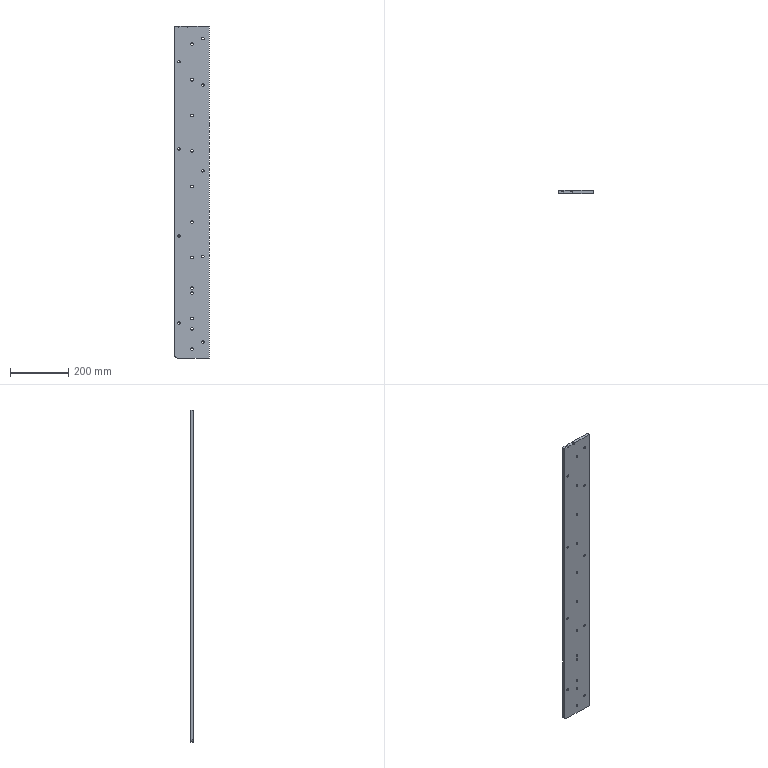Part | STEP file | 1 solid | 55 faces | box 120 x 10 x 1143 mm | volume 1358326 mm3 | cylinder 47 | plane 8 | commonest cylinder face diameters 9 x24 8.4 x10 8.5 x8 7 x4 20 x1